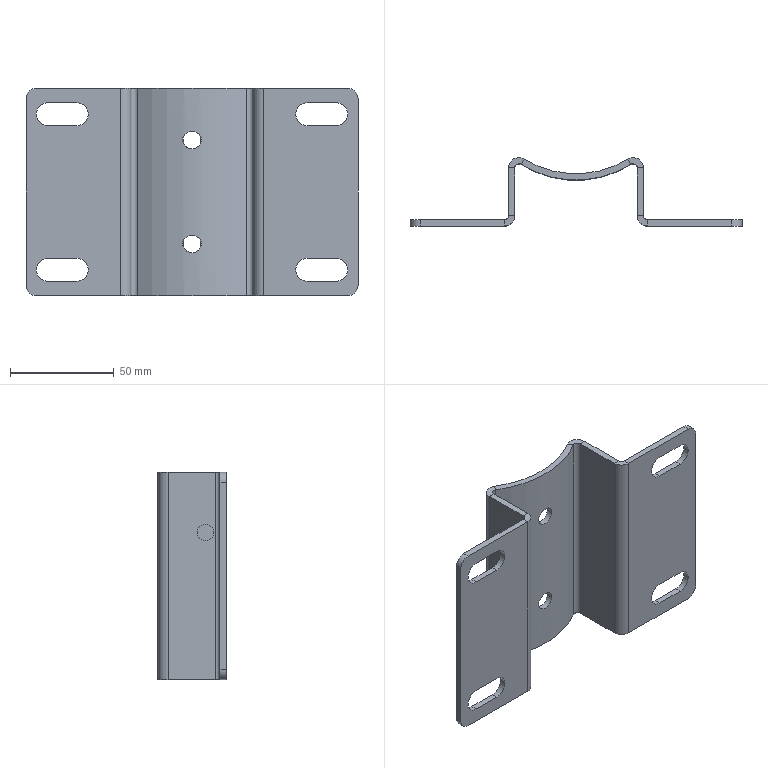Part | STEP file | 5090601 | 1 solid | 61 faces | box 160 x 33 x 100 mm | volume 61520 mm3 | plane 36 | cylinder 23 | spline 2 | commonest cylinder face diameters 11 x8 10 x6 3.946 x2 4 x2 9.946 x2 8 x1